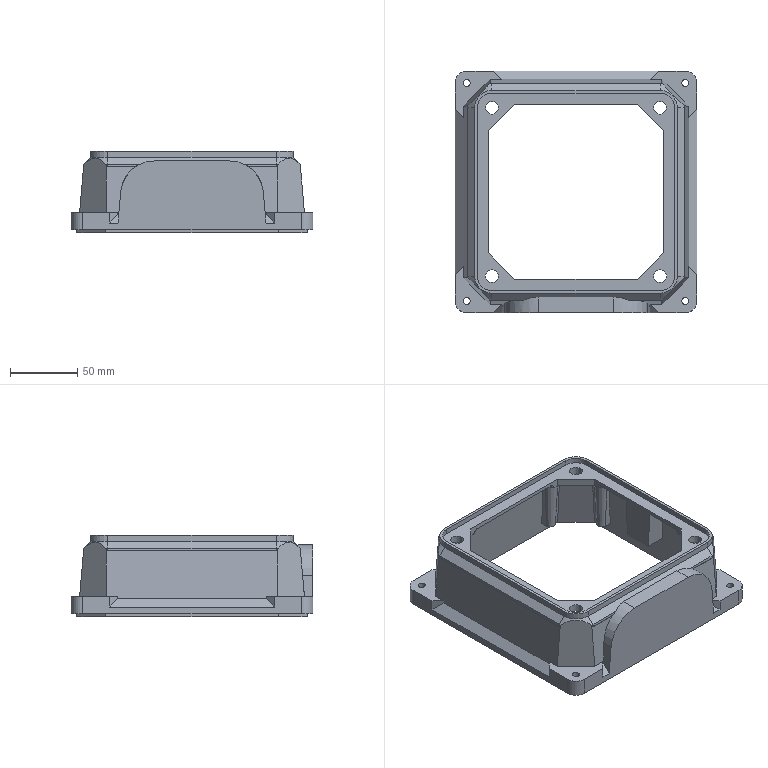Part | STEP file | Input 98 | 1 solid | 216 faces | box 179.5 x 179.5 x 60.5 mm | volume 241417 mm3 | plane 154 | cylinder 40 | cone 22 | commonest cylinder face diameters 4 x8 5.188 x8 9.5 x8 17.5 x4 21.5 x4 25.5 x4